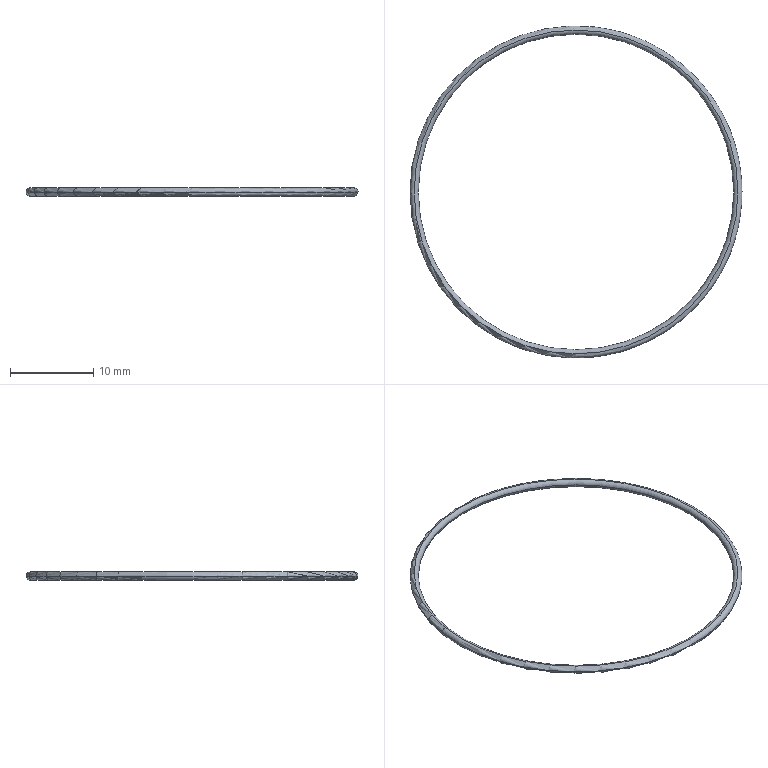Part | NX | features DATUM_CSYS 2, BLEND 1, EXTRUDE 1, SKETCH 1 | 1 solid | 4 faces | box 40 x 40 x 1 mm | volume 96.229 mm3 | torus 4
STEP:
#1=CARTESIAN_POINT('',(-19.,0.,0.5));
#2=VERTEX_POINT('',#1);
#3=CARTESIAN_POINT('',(0.,0.,0.5));
#4=DIRECTION('',(0.,0.,-1.));
#5=DIRECTION('',(-1.,0.,0.));
#6=AXIS2_PLACEMENT_3D('',#3,#4,#5);
#7=CIRCLE('',#6,19.);
#8=EDGE_CURVE('',#2,#2,#7,.F.);
#9=ORIENTED_EDGE('',*,*,#8,.F.);
#10=EDGE_LOOP('',(#9));
#11=FACE_BOUND('',#10,.T.);
#12=CARTESIAN_POINT('',(-19.5,0.,1.));
#13=VERTEX_POINT('',#12);
#14=CARTESIAN_POINT('',(0.,0.,1.));
#15=DIRECTION('',(0.,0.,-1.));
#16=DIRECTION('',(-1.,0.,0.));
#17=AXIS2_PLACEMENT_3D('',#14,#15,#16);
#18=CIRCLE('',#17,19.5);
#19=EDGE_CURVE('',#13,#13,#18,.T.);
#20=ORIENTED_EDGE('',*,*,#19,.F.);
#21=EDGE_LOOP('',(#20));
#22=FACE_BOUND('',#21,.T.);
#23=CARTESIAN_POINT('',(0.,0.,0.5));
#24=DIRECTION('',(0.,0.,-1.));
#25=DIRECTION('',(-1.,0.,0.));
#26=AXIS2_PLACEMENT_3D('',#23,#24,#25);
#27=TOROIDAL_SURFACE('',#26,19.5,0.5);
#28=ADVANCED_FACE('',(#11,#22),#27,.T.);
#29=ORIENTED_EDGE('',*,*,#19,.T.);
#30=EDGE_LOOP('',(#29));
#31=FACE_BOUND('',#30,.T.);
#32=CARTESIAN_POINT('',(-20.,0.,0.5));
#33=VERTEX_POINT('',#32);
#34=CARTESIAN_POINT('',(0.,0.,0.5));
#35=DIRECTION('',(0.,0.,-1.));
#36=DIRECTION('',(-1.,0.,0.));
#37=AXIS2_PLACEMENT_3D('',#34,#35,#36);
#38=CIRCLE('',#37,20.);
#39=EDGE_CURVE('',#33,#33,#38,.T.);
#40=ORIENTED_EDGE('',*,*,#39,.F.);
#41=EDGE_LOOP('',(#40));
#42=FACE_BOUND('',#41,.T.);
#43=CARTESIAN_POINT('',(0.,0.,0.5));
#44=DIRECTION('',(0.,0.,-1.));
#45=DIRECTION('',(-1.,0.,0.));
#46=AXIS2_PLACEMENT_3D('',#43,#44,#45);
#47=TOROIDAL_SURFACE('',#46,19.5,0.5);
#48=ADVANCED_FACE('',(#31,#42),#47,.T.);
#49=ORIENTED_EDGE('',*,*,#8,.T.);
#50=EDGE_LOOP('',(#49));
#51=FACE_BOUND('',#50,.T.);
#52=CARTESIAN_POINT('',(-19.5,0.,0.));
#53=VERTEX_POINT('',#52);
#54=CARTESIAN_POINT('',(0.,0.,0.));
#55=DIRECTION('',(0.,0.,-1.));
#56=DIRECTION('',(-1.,0.,0.));
#57=AXIS2_PLACEMENT_3D('',#54,#55,#56);
#58=CIRCLE('',#57,19.5);
#59=EDGE_CURVE('',#53,#53,#58,.F.);
#60=ORIENTED_EDGE('',*,*,#59,.F.);
#61=EDGE_LOOP('',(#60));
#62=FACE_BOUND('',#61,.T.);
#63=CARTESIAN_POINT('',(0.,0.,0.5));
#64=DIRECTION('',(0.,0.,-1.));
#65=DIRECTION('',(-1.,0.,0.));
#66=AXIS2_PLACEMENT_3D('',#63,#64,#65);
#67=TOROIDAL_SURFACE('',#66,19.5,0.5);
#68=ADVANCED_FACE('',(#51,#62),#67,.T.);
#69=ORIENTED_EDGE('',*,*,#39,.T.);
#70=EDGE_LOOP('',(#69));
#71=FACE_BOUND('',#70,.T.);
#72=ORIENTED_EDGE('',*,*,#59,.T.);
#73=EDGE_LOOP('',(#72));
#74=FACE_BOUND('',#73,.T.);
#75=CARTESIAN_POINT('',(0.,0.,0.5));
#76=DIRECTION('',(0.,0.,-1.));
#77=DIRECTION('',(-1.,0.,0.));
#78=AXIS2_PLACEMENT_3D('',#75,#76,#77);
#79=TOROIDAL_SURFACE('',#78,19.5,0.5);
#80=ADVANCED_FACE('',(#71,#74),#79,.T.);
#81=CLOSED_SHELL('',(#28,#48,#68,#80));
#82=MANIFOLD_SOLID_BREP('',#81);
#83=(LENGTH_UNIT()NAMED_UNIT(*)SI_UNIT(.MILLI.,.METRE.));
#84=UNCERTAINTY_MEASURE_WITH_UNIT(LENGTH_MEASURE(0.00001),#83,'','');
#85=(NAMED_UNIT(*)PLANE_ANGLE_UNIT()SI_UNIT($,.RADIAN.));
#86=(NAMED_UNIT(*)SI_UNIT($,.STERADIAN.)SOLID_ANGLE_UNIT());
#87=(GEOMETRIC_REPRESENTATION_CONTEXT(3)GLOBAL_UNCERTAINTY_ASSIGNED_CONTEXT((#84))GLOBAL_UNIT_ASSIGNED_CONTEXT((#83,#85,#86))REPRESENTATION_CONTEXT('',''));
#88=ADVANCED_BREP_SHAPE_REPRESENTATION('',(#82),#87);